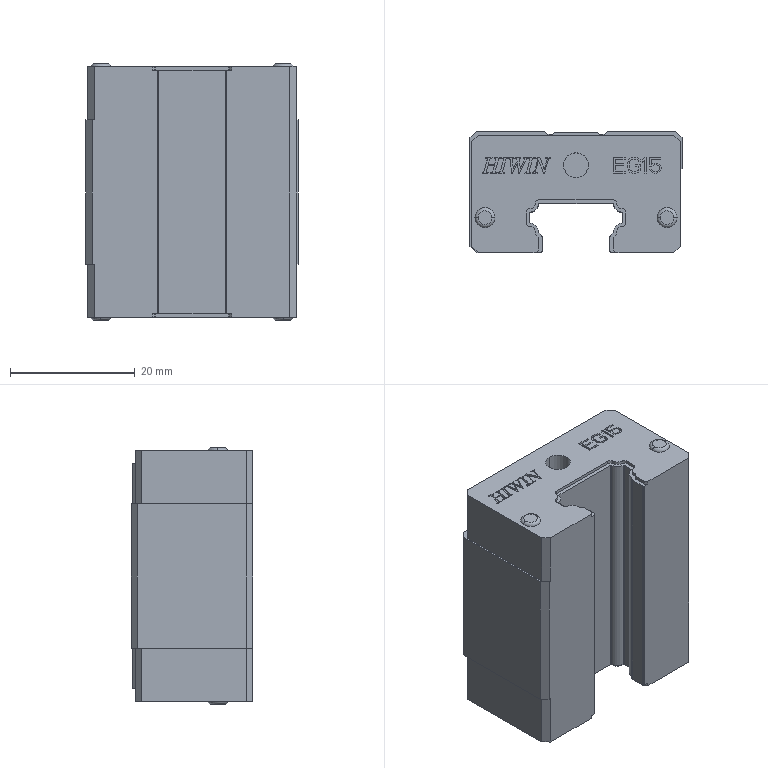Part | SolidWorks | features BaseBody 1 | 1 solid | 393 faces | box 34 x 19.5 x 41.1 mm | volume 21445 mm3 | plane 261 | cylinder 60 | spline 60 | torus 8 | cone 4 | commonest cylinder face diameters 1.6 x16 2.1 x12 0.46 x8 0.6 x4 0.74 x4 3 x4